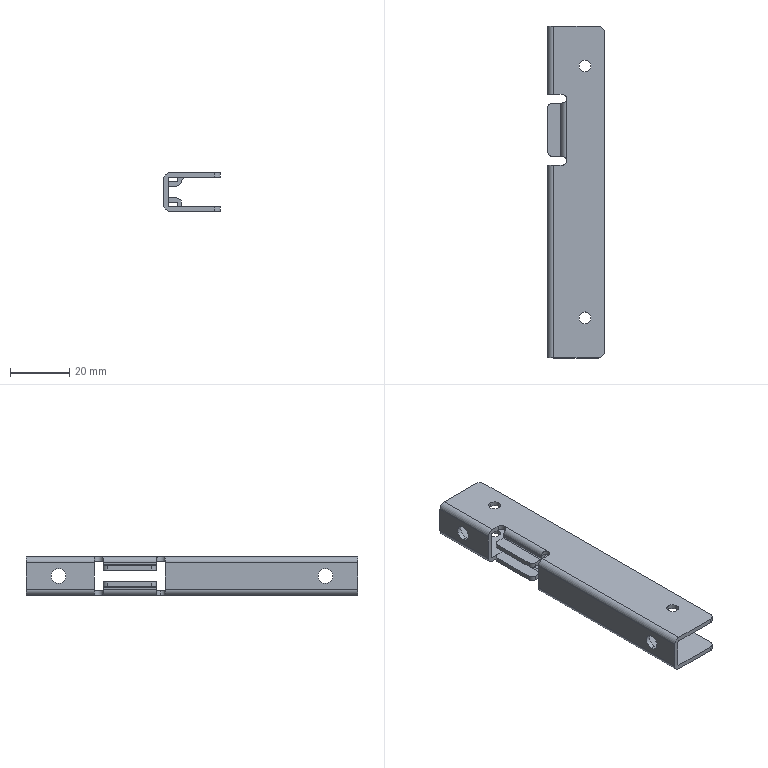Part | SolidWorks | features BaseBody 1 | 1 solid | 68 faces | box 19 x 112 x 13 mm | volume 7436 mm3 | cylinder 41 | plane 27 | commonest cylinder face diameters 4 x16 3 x9 3.6 x5 1 x4 5 x4 0.6 x3